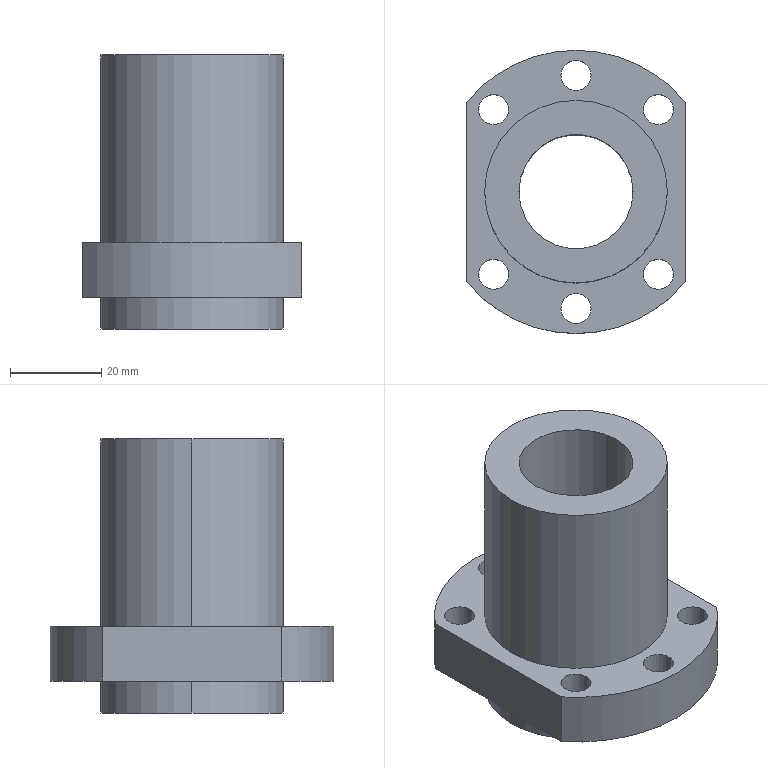Part | STEP file | ball screw nut-SFS02525-1.8 | 1 solid | 26 faces | box 48 x 62 x 60 mm | volume 60127 mm3 | cylinder 20 | plane 6 | commonest cylinder face diameters 6.6 x12 40 x4 25 x2 62 x2